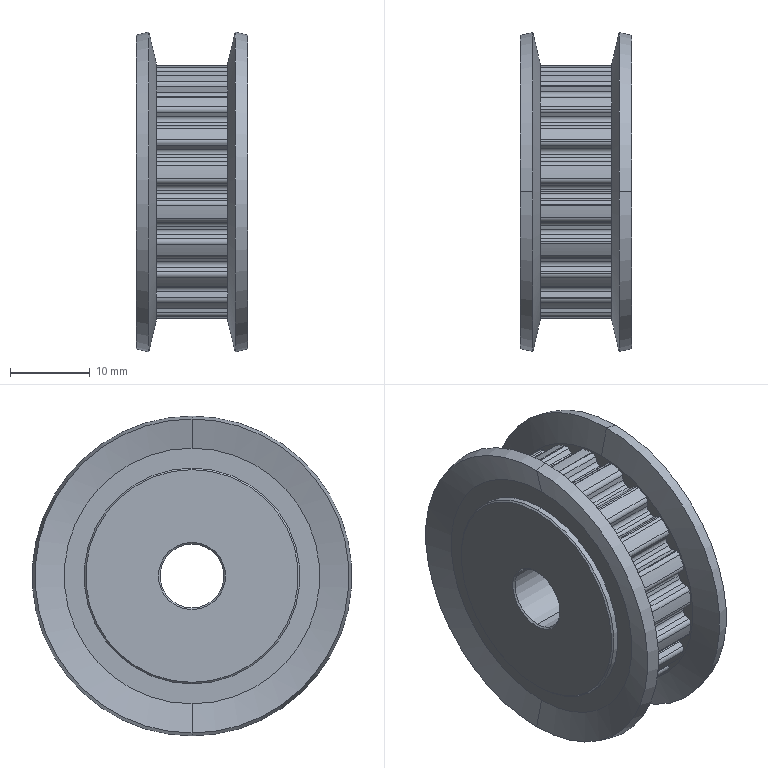Part | SolidWorks | features BaseBody 1 | 1 solid | 205 faces | box 14 x 40 x 40 mm | volume 10988 mm3 | cylinder 143 | plane 46 | cone 16 | commonest cylinder face diameters 1.22 x96 29.03 x21 31.83 x20 27 x4 8 x2